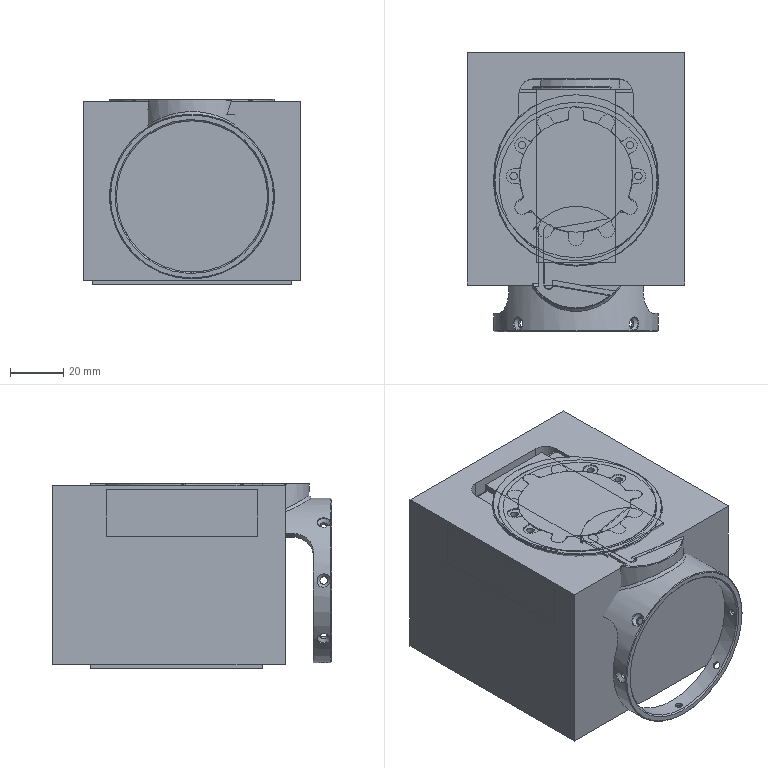NC program | NX | posted with a generic post | part box 82 x 105.2 x 70 mm
Whole program:
N10 G17 G21 G94 G90
(单向轮廓精光_4_COPY , TOOL : D10加长刀)
N12 T10 M6
N14 G53
N16 G17 G0 G90 X6.342 Y-17.835 B0. C0. S6500 M3
N18 G43 Z40. H10
N20 Z-51.
N22 G94 G1 Z-54. F700.
N24 G41 X9.003 Y-22.444 D30
N26 G3 X11.735 Y-23.176 R2.
N28 X20.326 Y8.885 R23.47
N30 X11.735 Y-23.176 R-23.47
N32 X12.165 Y-22.921 R23.47
N34 X12.839 Y-20.174 R2.
N36 G40
N38 G1 X12.735 Y-20.003
N40 X8.913 Y-22.288
N42 G41 X9.013 Y-22.461
N44 G3 X11.745 Y-23.193 R2.
N46 X20.343 Y8.895 R23.49
N48 X11.745 Y-23.193 R-23.49
N50 X12.175 Y-22.938 R23.49
N52 X12.849 Y-20.191 R2.
N54 G40
N56 G1 X12.745 Y-20.02
N58 X8.918 Y-22.296
N60 G41 X9.018 Y-22.47
N62 G3 X11.75 Y-23.202 R2.
N64 X20.352 Y8.9 R23.5
N66 X11.75 Y-23.202 R-23.5
N68 X12.18 Y-22.947 R23.5
N70 X12.854 Y-20.2 R2.
N72 G1 X10.199 Y-15.82
N74 G40
N76 X10.096 Y-15.649
N78 Z-51.
N80 G0 Z40.
(单向轮廓精光_4_COPY_COPY , TOOL : D10加长刀)
N82 X-12.6 Y-8.41
N84 Z-53.
N86 G1 Z-56.
N88 G41 X-17.124 Y-11.254
N90 G3 X-17.753 Y-14.012 R2.
N92 X11.162 Y-20.603 R20.97
N94 X-17.753 Y-14.012 R-20.97
N96 X-17.481 Y-14.432 R20.97
N98 X-14.71 Y-14.995 R2.
N100 G40
N102 G1 X-14.543 Y-14.884
N104 X-16.972 Y-11.158
N106 G41 X-17.141 Y-11.265
N108 G3 X-17.77 Y-14.022 R2.
N110 X11.172 Y-20.62 R20.99
N112 X-17.77 Y-14.022 R-20.99
N114 X-17.498 Y-14.442 R20.99
N116 X-14.727 Y-15.005 R2.
N118 G40
N120 G1 X-14.56 Y-14.895
N122 X-16.98 Y-11.164
N124 G41 X-17.149 Y-11.27
N126 G3 X-17.778 Y-14.028 R2.
N128 X11.178 Y-20.628 R21.
N130 X-17.778 Y-14.028 R-21.
N132 X-17.507 Y-14.448 R21.
N134 X-14.735 Y-15.011 R2.
N136 G1 X-10.447 Y-12.17
N138 G40
N140 X-10.28 Y-12.059
N142 Z-53.
N144 G0 Z40.
N146 M5
N148 M2